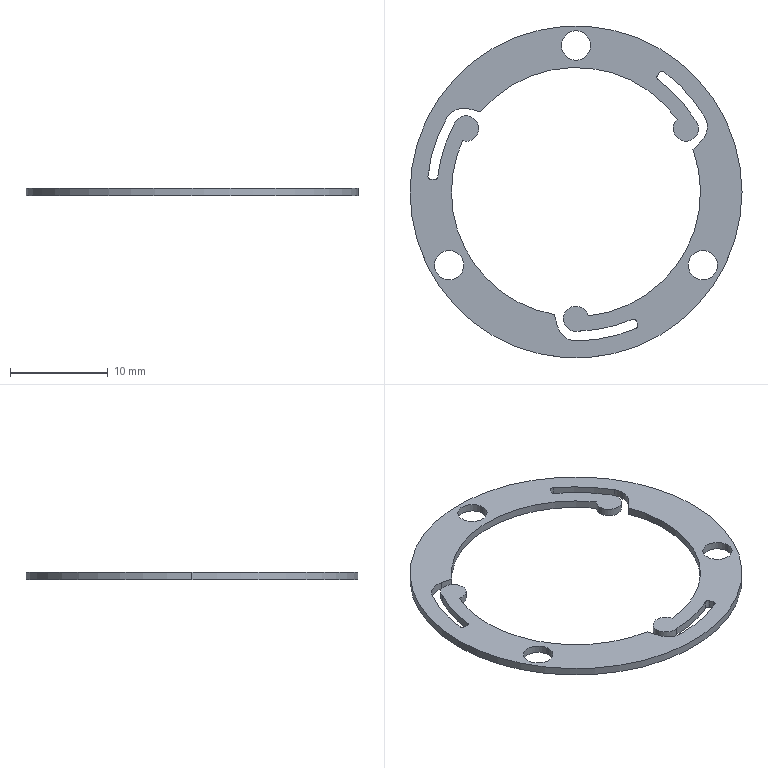Part | SolidWorks | features Fillet 3, ICE 3, CirPattern 2, DelFace 1, Extrusion 1 | 1 solid | 43 faces | box 34 x 34 x 0.8 mm | volume 283.992 mm3 | cylinder 35 | plane 8 | commonest cylinder face diameters 0.6 x7 2.6 x6 3 x6 4 x4 25.5 x4 28.5 x3
STEP:
#1=CARTESIAN_POINT('',(-17.,0.,0.));
#2=VERTEX_POINT('',#1);
#3=CARTESIAN_POINT('',(17.,0.,0.));
#4=VERTEX_POINT('',#3);
#5=CARTESIAN_POINT('',(0.,0.,0.));
#6=DIRECTION('',(0.,0.,-1.));
#7=DIRECTION('',(1.,0.,0.));
#8=AXIS2_PLACEMENT_3D('',#5,#6,#7);
#9=CIRCLE('',#8,17.);
#10=EDGE_CURVE('',#2,#4,#9,.T.);
#11=ORIENTED_EDGE('',*,*,#10,.F.);
#12=CARTESIAN_POINT('',(-17.,0.,0.8));
#13=VERTEX_POINT('',#12);
#14=CARTESIAN_POINT('',(-17.,0.,-26.154));
#15=DIRECTION('',(0.,0.,1.));
#16=VECTOR('',#15,1000.);
#17=LINE('',#14,#16);
#18=EDGE_CURVE('',#2,#13,#17,.T.);
#19=ORIENTED_EDGE('',*,*,#18,.T.);
#20=CARTESIAN_POINT('',(17.,0.,0.8));
#21=VERTEX_POINT('',#20);
#22=CARTESIAN_POINT('',(0.,0.,0.8));
#23=DIRECTION('',(0.,0.,1.));
#24=DIRECTION('',(1.,0.,0.));
#25=AXIS2_PLACEMENT_3D('',#22,#23,#24);
#26=CIRCLE('',#25,17.);
#27=EDGE_CURVE('',#21,#13,#26,.T.);
#28=ORIENTED_EDGE('',*,*,#27,.F.);
#29=CARTESIAN_POINT('',(17.,0.,-26.154));
#30=DIRECTION('',(0.,0.,1.));
#31=VECTOR('',#30,1000.);
#32=LINE('',#29,#31);
#33=EDGE_CURVE('',#4,#21,#32,.T.);
#34=ORIENTED_EDGE('',*,*,#33,.F.);
#35=EDGE_LOOP('',(#11,#19,#28,#34));
#36=FACE_OUTER_BOUND('',#35,.T.);
#37=CARTESIAN_POINT('',(0.,0.,-26.154));
#38=DIRECTION('',(0.,0.,1.));
#39=DIRECTION('',(1.,0.,0.));
#40=AXIS2_PLACEMENT_3D('',#37,#38,#39);
#41=CYLINDRICAL_SURFACE('',#40,17.);
#42=ADVANCED_FACE('',(#36),#41,.T.);
#43=CARTESIAN_POINT('',(6.345,-13.673,0.));
#44=VERTEX_POINT('',#43);
#45=CARTESIAN_POINT('',(6.317,-13.547,0.));
#46=VERTEX_POINT('',#45);
#47=CARTESIAN_POINT('',(6.045,-13.673,0.));
#48=DIRECTION('',(0.,0.,1.));
#49=DIRECTION('',(1.,0.,0.));
#50=AXIS2_PLACEMENT_3D('',#47,#48,#49);
#51=CIRCLE('',#50,0.3);
#52=EDGE_CURVE('',#44,#46,#51,.T.);
#53=ORIENTED_EDGE('',*,*,#52,.F.);
#54=CARTESIAN_POINT('',(6.345,-13.673,0.8));
#55=VERTEX_POINT('',#54);
#56=CARTESIAN_POINT('',(6.345,-13.673,-9.068));
#57=DIRECTION('',(0.,0.,1.));
#58=VECTOR('',#57,1000.);
#59=LINE('',#56,#58);
#60=EDGE_CURVE('',#44,#55,#59,.T.);
#61=ORIENTED_EDGE('',*,*,#60,.T.);
#62=CARTESIAN_POINT('',(6.317,-13.547,0.8));
#63=VERTEX_POINT('',#62);
#64=CARTESIAN_POINT('',(6.045,-13.673,0.8));
#65=DIRECTION('',(0.,0.,-1.));
#66=DIRECTION('',(1.,0.,0.));
#67=AXIS2_PLACEMENT_3D('',#64,#65,#66);
#68=CIRCLE('',#67,0.3);
#69=EDGE_CURVE('',#63,#55,#68,.T.);
#70=ORIENTED_EDGE('',*,*,#69,.F.);
#71=CARTESIAN_POINT('',(6.317,-13.547,0.8));
#72=DIRECTION('',(0.,0.,1.));
#73=VECTOR('',#72,1000.);
#74=LINE('',#71,#73);
#75=EDGE_CURVE('',#46,#63,#74,.T.);
#76=ORIENTED_EDGE('',*,*,#75,.F.);
#77=EDGE_LOOP('',(#53,#61,#70,#76));
#78=FACE_OUTER_BOUND('',#77,.T.);
#79=CARTESIAN_POINT('',(6.045,-13.673,-9.068));
#80=DIRECTION('',(0.,0.,1.));
#81=DIRECTION('',(1.,0.,0.));
#82=AXIS2_PLACEMENT_3D('',#79,#80,#81);
#83=CYLINDRICAL_SURFACE('',#82,0.3);
#84=ADVANCED_FACE('',(#78),#83,.F.);
#85=CARTESIAN_POINT('',(-9.958,6.5,0.));
#86=VERTEX_POINT('',#85);
#87=CARTESIAN_POINT('',(-11.619,5.251,0.));
#88=VERTEX_POINT('',#87);
#89=CARTESIAN_POINT('',(-11.258,6.5,0.));
#90=DIRECTION('',(0.,0.,-1.));
#91=DIRECTION('',(1.,0.,0.));
#92=AXIS2_PLACEMENT_3D('',#89,#90,#91);
#93=CIRCLE('',#92,1.3);
#94=EDGE_CURVE('',#86,#88,#93,.T.);
#95=ORIENTED_EDGE('',*,*,#94,.F.);
#96=CARTESIAN_POINT('',(-9.958,6.5,0.8));
#97=VERTEX_POINT('',#96);
#98=CARTESIAN_POINT('',(-9.958,6.5,-3.677));
#99=DIRECTION('',(0.,0.,1.));
#100=VECTOR('',#99,1000.);
#101=LINE('',#98,#100);
#102=EDGE_CURVE('',#86,#97,#101,.T.);
#103=ORIENTED_EDGE('',*,*,#102,.T.);
#104=CARTESIAN_POINT('',(-11.619,5.251,0.8));
#105=VERTEX_POINT('',#104);
#106=CARTESIAN_POINT('',(-11.258,6.5,0.8));
#107=DIRECTION('',(0.,0.,1.));
#108=DIRECTION('',(-0.5,0.866,0.));
#109=AXIS2_PLACEMENT_3D('',#106,#107,#108);
#110=CIRCLE('',#109,1.3);
#111=EDGE_CURVE('',#105,#97,#110,.T.);
#112=ORIENTED_EDGE('',*,*,#111,.F.);
#113=CARTESIAN_POINT('',(-11.619,5.251,0.4));
#114=DIRECTION('',(0.,0.,-1.));
#115=VECTOR('',#114,1000.);
#116=LINE('',#113,#115);
#117=EDGE_CURVE('',#105,#88,#116,.T.);
#118=ORIENTED_EDGE('',*,*,#117,.T.);
#119=EDGE_LOOP('',(#95,#103,#112,#118));
#120=FACE_OUTER_BOUND('',#119,.T.);
#121=CARTESIAN_POINT('',(-11.258,6.5,-3.677));
#122=DIRECTION('',(0.,0.,1.));
#123=DIRECTION('',(1.,0.,0.));
#124=AXIS2_PLACEMENT_3D('',#121,#122,#123);
#125=CYLINDRICAL_SURFACE('',#124,1.3);
#126=ADVANCED_FACE('',(#120),#125,.T.);
#127=CARTESIAN_POINT('',(9.958,6.5,0.));
#128=VERTEX_POINT('',#127);
#129=CARTESIAN_POINT('',(10.357,7.437,0.));
#130=VERTEX_POINT('',#129);
#131=CARTESIAN_POINT('',(11.258,6.5,0.));
#132=DIRECTION('',(0.,0.,-1.));
#133=DIRECTION('',(1.,0.,0.));
#134=AXIS2_PLACEMENT_3D('',#131,#132,#133);
#135=CIRCLE('',#134,1.3);
#136=EDGE_CURVE('',#128,#130,#135,.T.);
#137=ORIENTED_EDGE('',*,*,#136,.F.);
#138=CARTESIAN_POINT('',(9.958,6.5,0.8));
#139=VERTEX_POINT('',#138);
#140=CARTESIAN_POINT('',(9.958,6.5,-3.677));
#141=DIRECTION('',(0.,0.,1.));
#142=VECTOR('',#141,1000.);
#143=LINE('',#140,#142);
#144=EDGE_CURVE('',#128,#139,#143,.T.);
#145=ORIENTED_EDGE('',*,*,#144,.T.);
#146=CARTESIAN_POINT('',(10.357,7.437,0.8));
#147=VERTEX_POINT('',#146);
#148=CARTESIAN_POINT('',(11.258,6.5,0.8));
#149=DIRECTION('',(0.,0.,1.));
#150=DIRECTION('',(1.,0.,0.));
#151=AXIS2_PLACEMENT_3D('',#148,#149,#150);
#152=CIRCLE('',#151,1.3);
#153=EDGE_CURVE('',#147,#139,#152,.T.);
#154=ORIENTED_EDGE('',*,*,#153,.F.);
#155=CARTESIAN_POINT('',(10.357,7.437,0.4));
#156=DIRECTION('',(0.,0.,-1.));
#157=VECTOR('',#156,1000.);
#158=LINE('',#155,#157);
#159=EDGE_CURVE('',#147,#130,#158,.T.);
#160=ORIENTED_EDGE('',*,*,#159,.T.);
#161=EDGE_LOOP('',(#137,#145,#154,#160));
#162=FACE_OUTER_BOUND('',#161,.T.);
#163=CARTESIAN_POINT('',(11.258,6.5,-3.677));
#164=DIRECTION('',(0.,0.,1.));
#165=DIRECTION('',(1.,0.,0.));
#166=AXIS2_PLACEMENT_3D('',#163,#164,#165);
#167=CYLINDRICAL_SURFACE('',#166,1.3);
#168=ADVANCED_FACE('',(#162),#167,.T.);
#169=ORIENTED_EDGE('',*,*,#144,.F.);
#170=CARTESIAN_POINT('',(12.558,6.5,0.));
#171=VERTEX_POINT('',#170);
#172=CARTESIAN_POINT('',(11.258,6.5,0.));
#173=DIRECTION('',(0.,0.,-1.));
#174=DIRECTION('',(1.,0.,0.));
#175=AXIS2_PLACEMENT_3D('',#172,#173,#174);
#176=CIRCLE('',#175,1.3);
#177=EDGE_CURVE('',#171,#128,#176,.T.);
#178=ORIENTED_EDGE('',*,*,#177,.F.);
#179=CARTESIAN_POINT('',(12.558,6.5,0.8));
#180=VERTEX_POINT('',#179);
#181=CARTESIAN_POINT('',(12.558,6.5,-3.677));
#182=DIRECTION('',(0.,0.,1.));
#183=VECTOR('',#182,1000.);
#184=LINE('',#181,#183);
#185=EDGE_CURVE('',#171,#180,#184,.T.);
#186=ORIENTED_EDGE('',*,*,#185,.T.);
#187=CARTESIAN_POINT('',(11.258,6.5,0.8));
#188=DIRECTION('',(0.,0.,1.));
#189=DIRECTION('',(1.,0.,0.));
#190=AXIS2_PLACEMENT_3D('',#187,#188,#189);
#191=CIRCLE('',#190,1.3);
#192=EDGE_CURVE('',#139,#180,#191,.T.);
#193=ORIENTED_EDGE('',*,*,#192,.F.);
#194=EDGE_LOOP('',(#169,#178,#186,#193));
#195=FACE_OUTER_BOUND('',#194,.T.);
#196=CARTESIAN_POINT('',(11.258,6.5,-3.677));
#197=DIRECTION('',(0.,0.,1.));
#198=DIRECTION('',(1.,0.,0.));
#199=AXIS2_PLACEMENT_3D('',#196,#197,#198);
#200=CYLINDRICAL_SURFACE('',#199,1.3);
#201=ADVANCED_FACE('',(#195),#200,.T.);
#202=CARTESIAN_POINT('',(13.454,6.662,0.));
#203=VERTEX_POINT('',#202);
#204=CARTESIAN_POINT('',(13.182,7.667,0.));
#205=VERTEX_POINT('',#204);
#206=CARTESIAN_POINT('',(11.454,6.662,0.));
#207=DIRECTION('',(0.,0.,1.));
#208=DIRECTION('',(1.,0.,0.));
#209=AXIS2_PLACEMENT_3D('',#206,#207,#208);
#210=CIRCLE('',#209,2.);
#211=EDGE_CURVE('',#203,#205,#210,.T.);
#212=ORIENTED_EDGE('',*,*,#211,.F.);
#213=CARTESIAN_POINT('',(13.454,6.662,0.8));
#214=VERTEX_POINT('',#213);
#215=CARTESIAN_POINT('',(13.454,6.662,-9.944));
#216=DIRECTION('',(0.,0.,1.));
#217=VECTOR('',#216,1000.);
#218=LINE('',#215,#217);
#219=EDGE_CURVE('',#203,#214,#218,.T.);
#220=ORIENTED_EDGE('',*,*,#219,.T.);
#221=CARTESIAN_POINT('',(13.182,7.667,0.8));
#222=VERTEX_POINT('',#221);
#223=CARTESIAN_POINT('',(11.454,6.662,0.8));
#224=DIRECTION('',(0.,0.,-1.));
#225=DIRECTION('',(1.,0.,0.));
#226=AXIS2_PLACEMENT_3D('',#223,#224,#225);
#227=CIRCLE('',#226,2.);
#228=EDGE_CURVE('',#222,#214,#227,.T.);
#229=ORIENTED_EDGE('',*,*,#228,.F.);
#230=CARTESIAN_POINT('',(13.182,7.667,-9.944));
#231=DIRECTION('',(0.,0.,1.));
#232=VECTOR('',#231,1000.);
#233=LINE('',#230,#232);
#234=EDGE_CURVE('',#205,#222,#233,.T.);
#235=ORIENTED_EDGE('',*,*,#234,.F.);
#236=EDGE_LOOP('',(#212,#220,#229,#235));
#237=FACE_OUTER_BOUND('',#236,.T.);
#238=CARTESIAN_POINT('',(11.454,6.662,-9.944));
#239=DIRECTION('',(0.,0.,1.));
#240=DIRECTION('',(1.,0.,0.));
#241=AXIS2_PLACEMENT_3D('',#238,#239,#240);
#242=CYLINDRICAL_SURFACE('',#241,2.);
#243=ADVANCED_FACE('',(#237),#242,.F.);
#244=CARTESIAN_POINT('',(-14.49,-7.5,0.8));
#245=VERTEX_POINT('',#244);
#246=CARTESIAN_POINT('',(-11.49,-7.5,0.8));
#247=VERTEX_POINT('',#246);
#248=CARTESIAN_POINT('',(-12.99,-7.5,0.8));
#249=DIRECTION('',(0.,0.,1.));
#250=DIRECTION('',(1.,0.,0.));
#251=AXIS2_PLACEMENT_3D('',#248,#249,#250);
#252=CIRCLE('',#251,1.5);
#253=EDGE_CURVE('',#245,#247,#252,.T.);
#254=ORIENTED_EDGE('',*,*,#253,.T.);
#255=CARTESIAN_POINT('',(-11.49,-7.5,0.));
#256=VERTEX_POINT('',#255);
#257=CARTESIAN_POINT('',(-11.49,-7.5,0.8));
#258=DIRECTION('',(0.,0.,-1.));
#259=VECTOR('',#258,1000.);
#260=LINE('',#257,#259);
#261=EDGE_CURVE('',#247,#256,#260,.T.);
#262=ORIENTED_EDGE('',*,*,#261,.T.);
#263=CARTESIAN_POINT('',(-14.49,-7.5,0.));
#264=VERTEX_POINT('',#263);
#265=CARTESIAN_POINT('',(-12.99,-7.5,0.));
#266=DIRECTION('',(0.,0.,1.));
#267=DIRECTION('',(1.,0.,0.));
#268=AXIS2_PLACEMENT_3D('',#265,#266,#267);
#269=CIRCLE('',#268,1.5);
#270=EDGE_CURVE('',#264,#256,#269,.T.);
#271=ORIENTED_EDGE('',*,*,#270,.F.);
#272=CARTESIAN_POINT('',(-14.49,-7.5,0.8));
#273=DIRECTION('',(0.,0.,-1.));
#274=VECTOR('',#273,1000.);
#275=LINE('',#272,#274);
#276=EDGE_CURVE('',#245,#264,#275,.T.);
#277=ORIENTED_EDGE('',*,*,#276,.F.);
#278=EDGE_LOOP('',(#254,#262,#271,#277));
#279=FACE_OUTER_BOUND('',#278,.T.);
#280=CARTESIAN_POINT('',(-12.99,-7.5,0.8));
#281=DIRECTION('',(0.,0.,-1.));
#282=DIRECTION('',(-1.,0.,0.));
#283=AXIS2_PLACEMENT_3D('',#280,#281,#282);
#284=CYLINDRICAL_SURFACE('',#283,1.5);
#285=ADVANCED_FACE('',(#279),#284,.F.);
#286=CARTESIAN_POINT('',(11.49,-7.5,0.8));
#287=VERTEX_POINT('',#286);
#288=CARTESIAN_POINT('',(14.49,-7.5,0.8));
#289=VERTEX_POINT('',#288);
#290=CARTESIAN_POINT('',(12.99,-7.5,0.8));
#291=DIRECTION('',(0.,0.,1.));
#292=DIRECTION('',(1.,0.,0.));
#293=AXIS2_PLACEMENT_3D('',#290,#291,#292);
#294=CIRCLE('',#293,1.5);
#295=EDGE_CURVE('',#287,#289,#294,.T.);
#296=ORIENTED_EDGE('',*,*,#295,.T.);
#297=CARTESIAN_POINT('',(14.49,-7.5,0.));
#298=VERTEX_POINT('',#297);
#299=CARTESIAN_POINT('',(14.49,-7.5,0.8));
#300=DIRECTION('',(0.,0.,-1.));
#301=VECTOR('',#300,1000.);
#302=LINE('',#299,#301);
#303=EDGE_CURVE('',#289,#298,#302,.T.);
#304=ORIENTED_EDGE('',*,*,#303,.T.);
#305=CARTESIAN_POINT('',(11.49,-7.5,0.));
#306=VERTEX_POINT('',#305);
#307=CARTESIAN_POINT('',(12.99,-7.5,0.));
#308=DIRECTION('',(0.,0.,1.));
#309=DIRECTION('',(1.,0.,0.));
#310=AXIS2_PLACEMENT_3D('',#307,#308,#309);
#311=CIRCLE('',#310,1.5);
#312=EDGE_CURVE('',#306,#298,#311,.T.);
#313=ORIENTED_EDGE('',*,*,#312,.F.);
#314=CARTESIAN_POINT('',(11.49,-7.5,0.8));
#315=DIRECTION('',(0.,0.,-1.));
#316=VECTOR('',#315,1000.);
#317=LINE('',#314,#316);
#318=EDGE_CURVE('',#287,#306,#317,.T.);
#319=ORIENTED_EDGE('',*,*,#318,.F.);
#320=EDGE_LOOP('',(#296,#304,#313,#319));
#321=FACE_OUTER_BOUND('',#320,.T.);
#322=CARTESIAN_POINT('',(12.99,-7.5,0.8));
#323=DIRECTION('',(0.,0.,-1.));
#324=DIRECTION('',(-1.,0.,0.));
#325=AXIS2_PLACEMENT_3D('',#322,#323,#324);
#326=CYLINDRICAL_SURFACE('',#325,1.5);
#327=ADVANCED_FACE('',(#321),#326,.F.);
#328=CARTESIAN_POINT('',(-1.5,15.,0.8));
#329=VERTEX_POINT('',#328);
#330=CARTESIAN_POINT('',(1.5,15.,0.8));
#331=VERTEX_POINT('',#330);
#332=CARTESIAN_POINT('',(0.,15.,0.8));
#333=DIRECTION('',(0.,0.,1.));
#334=DIRECTION('',(1.,0.,0.));
#335=AXIS2_PLACEMENT_3D('',#332,#333,#334);
#336=CIRCLE('',#335,1.5);
#337=EDGE_CURVE('',#329,#331,#336,.T.);
#338=ORIENTED_EDGE('',*,*,#337,.T.);
#339=CARTESIAN_POINT('',(1.5,15.,0.));
#340=VERTEX_POINT('',#339);
#341=CARTESIAN_POINT('',(1.5,15.,0.8));
#342=DIRECTION('',(0.,0.,-1.));
#343=VECTOR('',#342,1000.);
#344=LINE('',#341,#343);
#345=EDGE_CURVE('',#331,#340,#344,.T.);
#346=ORIENTED_EDGE('',*,*,#345,.T.);
#347=CARTESIAN_POINT('',(-1.5,15.,0.));
#348=VERTEX_POINT('',#347);
#349=CARTESIAN_POINT('',(0.,15.,0.));
#350=DIRECTION('',(0.,0.,1.));
#351=DIRECTION('',(1.,0.,0.));
#352=AXIS2_PLACEMENT_3D('',#349,#350,#351);
#353=CIRCLE('',#352,1.5);
#354=EDGE_CURVE('',#348,#340,#353,.T.);
#355=ORIENTED_EDGE('',*,*,#354,.F.);
#356=CARTESIAN_POINT('',(-1.5,15.,0.8));
#357=DIRECTION('',(0.,0.,-1.));
#358=VECTOR('',#357,1000.);
#359=LINE('',#356,#358);
#360=EDGE_CURVE('',#329,#348,#359,.T.);
#361=ORIENTED_EDGE('',*,*,#360,.F.);
#362=EDGE_LOOP('',(#338,#346,#355,#361));
#363=FACE_OUTER_BOUND('',#362,.T.);
#364=CARTESIAN_POINT('',(0.,15.,0.8));
#365=DIRECTION('',(0.,0.,-1.));
#366=DIRECTION('',(-1.,0.,0.));
#367=AXIS2_PLACEMENT_3D('',#364,#365,#366);
#368=CYLINDRICAL_SURFACE('',#367,1.5);
#369=ADVANCED_FACE('',(#363),#368,.F.);
#370=CARTESIAN_POINT('',(-12.75,0.,0.8));
#371=VERTEX_POINT('',#370);
#372=CARTESIAN_POINT('',(0.,0.,0.8));
#373=DIRECTION('',(0.,0.,1.));
#374=DIRECTION('',(1.,0.,0.));
#375=AXIS2_PLACEMENT_3D('',#372,#373,#374);
#376=CIRCLE('',#375,12.75);
#377=EDGE_CURVE('',#105,#371,#376,.T.);
#378=ORIENTED_EDGE('',*,*,#377,.T.);
#379=CARTESIAN_POINT('',(-12.75,0.,0.));
#380=VERTEX_POINT('',#379);
#381=CARTESIAN_POINT('',(-12.75,0.,0.8));
#382=DIRECTION('',(0.,0.,-1.));
#383=VECTOR('',#382,1000.);
#384=LINE('',#381,#383);
#385=EDGE_CURVE('',#371,#380,#384,.T.);
#386=ORIENTED_EDGE('',*,*,#385,.T.);
#387=CARTESIAN_POINT('',(0.,0.,0.));
#388=DIRECTION('',(0.,0.,1.));
#389=DIRECTION('',(1.,0.,0.));
#390=AXIS2_PLACEMENT_3D('',#387,#388,#389);
#391=CIRCLE('',#390,12.75);
#392=EDGE_CURVE('',#88,#380,#391,.T.);
#393=ORIENTED_EDGE('',*,*,#392,.F.);
#394=ORIENTED_EDGE('',*,*,#117,.F.);
#395=EDGE_LOOP('',(#378,#386,#393,#394));
#396=FACE_OUTER_BOUND('',#395,.T.);
#397=CARTESIAN_POINT('',(0.,0.,0.8));
#398=DIRECTION('',(0.,0.,-1.));
#399=DIRECTION('',(-1.,0.,0.));
#400=AXIS2_PLACEMENT_3D('',#397,#398,#399);
#401=CYLINDRICAL_SURFACE('',#400,12.75);
#402=ADVANCED_FACE('',(#396),#401,.F.);
#403=CARTESIAN_POINT('',(1.262,-12.687,0.8));
#404=VERTEX_POINT('',#403);
#405=CARTESIAN_POINT('',(11.981,4.361,0.8));
#406=VERTEX_POINT('',#405);
#407=CARTESIAN_POINT('',(0.,0.,0.8));
#408=DIRECTION('',(0.,0.,1.));
#409=DIRECTION('',(1.,0.,0.));
#410=AXIS2_PLACEMENT_3D('',#407,#408,#409);
#411=CIRCLE('',#410,12.75);
#412=EDGE_CURVE('',#404,#406,#411,.T.);
#413=ORIENTED_EDGE('',*,*,#412,.F.);
#414=CARTESIAN_POINT('',(0.3738,-14.245,0.8));
#415=VERTEX_POINT('',#414);
#416=CARTESIAN_POINT('',(0.,-13.,0.8));
#417=DIRECTION('',(0.,0.,1.));
#418=DIRECTION('',(-0.5,-0.866,0.));
#419=AXIS2_PLACEMENT_3D('',#416,#417,#418);
#420=CIRCLE('',#419,1.3);
#421=EDGE_CURVE('',#404,#415,#420,.T.);
#422=ORIENTED_EDGE('',*,*,#421,.T.);
#423=CARTESIAN_POINT('',(5.755,-13.036,0.8));
#424=VERTEX_POINT('',#423);
#425=CARTESIAN_POINT('',(0.,0.,0.8));
#426=DIRECTION('',(0.,0.,-1.));
#427=DIRECTION('',(-0.5,-0.866,0.));
#428=AXIS2_PLACEMENT_3D('',#425,#426,#427);
#429=CIRCLE('',#428,14.25);
#430=EDGE_CURVE('',#424,#415,#429,.T.);
#431=ORIENTED_EDGE('',*,*,#430,.F.);
#432=CARTESIAN_POINT('',(6.148,-13.184,0.8));
#433=VERTEX_POINT('',#432);
#434=CARTESIAN_POINT('',(5.876,-13.311,0.8));
#435=DIRECTION('',(0.,0.,-1.));
#436=DIRECTION('',(1.,0.,0.));
#437=AXIS2_PLACEMENT_3D('',#434,#435,#436);
#438=CIRCLE('',#437,0.3);
#439=EDGE_CURVE('',#424,#433,#438,.T.);
#440=ORIENTED_EDGE('',*,*,#439,.T.);
#441=CARTESIAN_POINT('',(6.445,-13.821,0.8));
#442=DIRECTION('',(-0.4226,0.9063,0.));
#443=VECTOR('',#442,1000.);
#444=LINE('',#441,#443);
#445=EDGE_CURVE('',#63,#433,#444,.T.);
#446=ORIENTED_EDGE('',*,*,#445,.F.);
#447=ORIENTED_EDGE('',*,*,#69,.T.);
#448=CARTESIAN_POINT('',(6.166,-13.948,0.8));
#449=VERTEX_POINT('',#448);
#450=CARTESIAN_POINT('',(6.045,-13.673,0.8));
#451=DIRECTION('',(0.,0.,-1.));
#452=DIRECTION('',(1.,0.,0.));
#453=AXIS2_PLACEMENT_3D('',#450,#451,#452);
#454=CIRCLE('',#453,0.3);
#455=EDGE_CURVE('',#55,#449,#454,.T.);
#456=ORIENTED_EDGE('',*,*,#455,.T.);
#457=CARTESIAN_POINT('',(0.0488,-15.25,0.8));
#458=VERTEX_POINT('',#457);
#459=CARTESIAN_POINT('',(0.,0.,0.8));
#460=DIRECTION('',(0.,0.,1.));
#461=DIRECTION('',(-0.5,-0.866,0.));
#462=AXIS2_PLACEMENT_3D('',#459,#460,#461);
#463=CIRCLE('',#462,15.25);
#464=EDGE_CURVE('',#458,#449,#463,.T.);
#465=ORIENTED_EDGE('',*,*,#464,.F.);
#466=CARTESIAN_POINT('',(-1.889,-13.768,0.8));
#467=VERTEX_POINT('',#466);
#468=CARTESIAN_POINT('',(0.0424,-13.25,0.8));
#469=DIRECTION('',(0.,0.,-1.));
#470=DIRECTION('',(1.,0.,0.));
#471=AXIS2_PLACEMENT_3D('',#468,#469,#470);
#472=CIRCLE('',#471,2.);
#473=EDGE_CURVE('',#458,#467,#472,.T.);
#474=ORIENTED_EDGE('',*,*,#473,.T.);
#475=CARTESIAN_POINT('',(-2.214,-12.556,0.8));
#476=VERTEX_POINT('',#475);
#477=CARTESIAN_POINT('',(-2.214,-12.556,0.8));
#478=DIRECTION('',(0.2588,-0.9659,0.));
#479=VECTOR('',#478,1000.);
#480=LINE('',#477,#479);
#481=EDGE_CURVE('',#476,#467,#480,.T.);
#482=ORIENTED_EDGE('',*,*,#481,.F.);
#483=CARTESIAN_POINT('',(0.,0.,0.8));
#484=DIRECTION('',(0.,0.,1.));
#485=DIRECTION('',(1.,0.,0.));
#486=AXIS2_PLACEMENT_3D('',#483,#484,#485);
#487=CIRCLE('',#486,12.75);
#488=EDGE_CURVE('',#371,#476,#487,.T.);
#489=ORIENTED_EDGE('',*,*,#488,.F.);
#490=ORIENTED_EDGE('',*,*,#377,.F.);
#491=ORIENTED_EDGE('',*,*,#111,.T.);
#492=CARTESIAN_POINT('',(-12.524,6.799,0.8));
#493=VERTEX_POINT('',#492);
#494=CARTESIAN_POINT('',(-11.258,6.5,0.8));
#495=DIRECTION('',(0.,0.,1.));
#496=DIRECTION('',(-0.5,0.866,0.));
#497=AXIS2_PLACEMENT_3D('',#494,#495,#496);
#498=CIRCLE('',#497,1.3);
#499=EDGE_CURVE('',#97,#493,#498,.T.);
#500=ORIENTED_EDGE('',*,*,#499,.T.);
#501=CARTESIAN_POINT('',(-14.167,1.534,0.8));
#502=VERTEX_POINT('',#501);
#503=CARTESIAN_POINT('',(0.,0.,0.8));
#504=DIRECTION('',(0.,0.,-1.));
#505=DIRECTION('',(-0.5,0.866,0.));
#506=AXIS2_PLACEMENT_3D('',#503,#504,#505);
#507=CIRCLE('',#506,14.25);
#508=EDGE_CURVE('',#502,#493,#507,.T.);
#509=ORIENTED_EDGE('',*,*,#508,.F.);
#510=CARTESIAN_POINT('',(-14.492,1.268,0.8));
#511=VERTEX_POINT('',#510);
#512=CARTESIAN_POINT('',(-14.465,1.567,0.8));
#513=DIRECTION('',(0.,0.,-1.));
#514=DIRECTION('',(1.,0.,0.));
#515=AXIS2_PLACEMENT_3D('',#512,#513,#514);
#516=CIRCLE('',#515,0.3);
#517=EDGE_CURVE('',#502,#511,#516,.T.);
#518=ORIENTED_EDGE('',*,*,#517,.T.);
#519=CARTESIAN_POINT('',(-14.89,1.303,0.8));
#520=VERTEX_POINT('',#519);
#521=CARTESIAN_POINT('',(-15.192,1.329,0.8));
#522=DIRECTION('',(0.9962,-0.08716,0.));
#523=VECTOR('',#522,1000.);
#524=LINE('',#521,#523);
#525=EDGE_CURVE('',#520,#511,#524,.T.);
#526=ORIENTED_EDGE('',*,*,#525,.F.);
#527=CARTESIAN_POINT('',(-15.162,1.634,0.8));
#528=VERTEX_POINT('',#527);
#529=CARTESIAN_POINT('',(-14.864,1.602,0.8));
#530=DIRECTION('',(0.,0.,-1.));
#531=DIRECTION('',(1.,0.,0.));
#532=AXIS2_PLACEMENT_3D('',#529,#530,#531);
#533=CIRCLE('',#532,0.3);
#534=EDGE_CURVE('',#520,#528,#533,.T.);
#535=ORIENTED_EDGE('',*,*,#534,.T.);
#536=CARTESIAN_POINT('',(-13.231,7.583,0.8));
#537=VERTEX_POINT('',#536);
#538=CARTESIAN_POINT('',(0.,0.,0.8));
#539=DIRECTION('',(0.,0.,1.));
#540=DIRECTION('',(-0.5,0.866,0.));
#541=AXIS2_PLACEMENT_3D('',#538,#539,#540);
#542=CIRCLE('',#541,15.25);
#543=EDGE_CURVE('',#537,#528,#542,.T.);
#544=ORIENTED_EDGE('',*,*,#543,.F.);
#545=CARTESIAN_POINT('',(-10.978,8.52,0.8));
#546=VERTEX_POINT('',#545);
#547=CARTESIAN_POINT('',(-11.496,6.588,0.8));
#548=DIRECTION('',(0.,0.,-1.));
#549=DIRECTION('',(1.,0.,0.));
#550=AXIS2_PLACEMENT_3D('',#547,#548,#549);
#551=CIRCLE('',#550,2.);
#552=EDGE_CURVE('',#537,#546,#551,.T.);
#553=ORIENTED_EDGE('',*,*,#552,.T.);
#554=CARTESIAN_POINT('',(-9.767,8.196,0.8));
#555=VERTEX_POINT('',#554);
#556=CARTESIAN_POINT('',(-9.767,8.196,0.8));
#557=DIRECTION('',(-0.9659,0.2588,0.));
#558=VECTOR('',#557,1000.);
#559=LINE('',#556,#558);
#560=EDGE_CURVE('',#555,#546,#559,.T.);
#561=ORIENTED_EDGE('',*,*,#560,.F.);
#562=CARTESIAN_POINT('',(0.,0.,0.8));
#563=DIRECTION('',(0.,0.,1.));
#564=DIRECTION('',(1.,0.,0.));
#565=AXIS2_PLACEMENT_3D('',#562,#563,#564);
#566=CIRCLE('',#565,12.75);
#567=EDGE_CURVE('',#147,#555,#566,.T.);
#568=ORIENTED_EDGE('',*,*,#567,.F.);
#569=ORIENTED_EDGE('',*,*,#153,.T.);
#570=ORIENTED_EDGE('',*,*,#192,.T.);
#571=CARTESIAN_POINT('',(12.15,7.446,0.8));
#572=VERTEX_POINT('',#571);
#573=CARTESIAN_POINT('',(11.258,6.5,0.8));
#574=DIRECTION('',(0.,0.,1.));
#575=DIRECTION('',(1.,0.,0.));
#576=AXIS2_PLACEMENT_3D('',#573,#574,#575);
#577=CIRCLE('',#576,1.3);
#578=EDGE_CURVE('',#180,#572,#577,.T.);
#579=ORIENTED_EDGE('',*,*,#578,.T.);
#580=CARTESIAN_POINT('',(8.412,11.502,0.8));
#581=VERTEX_POINT('',#580);
#582=CARTESIAN_POINT('',(0.,0.,0.8));
#583=DIRECTION('',(0.,0.,-1.));
#584=DIRECTION('',(1.,0.,0.));
#585=AXIS2_PLACEMENT_3D('',#582,#583,#584);
#586=CIRCLE('',#585,14.25);
#587=EDGE_CURVE('',#581,#572,#586,.T.);
#588=ORIENTED_EDGE('',*,*,#587,.F.);
#589=CARTESIAN_POINT('',(8.344,11.916,0.8));
#590=VERTEX_POINT('',#589);
#591=CARTESIAN_POINT('',(8.59,11.744,0.8));
#592=DIRECTION('',(0.,0.,-1.));
#593=DIRECTION('',(1.,0.,0.));
#594=AXIS2_PLACEMENT_3D('',#591,#592,#593);
#595=CIRCLE('',#594,0.3);
#596=EDGE_CURVE('',#581,#590,#595,.T.);
#597=ORIENTED_EDGE('',*,*,#596,.T.);
#598=CARTESIAN_POINT('',(8.573,12.244,0.8));
#599=VERTEX_POINT('',#598);
#600=CARTESIAN_POINT('',(8.747,12.492,0.8));
#601=DIRECTION('',(-0.5736,-0.8192,0.));
#602=VECTOR('',#601,1000.);
#603=LINE('',#600,#602);
#604=EDGE_CURVE('',#599,#590,#603,.T.);
#605=ORIENTED_EDGE('',*,*,#604,.F.);
#606=CARTESIAN_POINT('',(8.996,12.314,0.8));
#607=VERTEX_POINT('',#606);
#608=CARTESIAN_POINT('',(8.819,12.072,0.8));
#609=DIRECTION('',(0.,0.,-1.));
#610=DIRECTION('',(1.,0.,0.));
#611=AXIS2_PLACEMENT_3D('',#608,#609,#610);
#612=CIRCLE('',#611,0.3);
#613=EDGE_CURVE('',#599,#607,#612,.T.);
#614=ORIENTED_EDGE('',*,*,#613,.T.);
#615=CARTESIAN_POINT('',(0.,0.,0.8));
#616=DIRECTION('',(0.,0.,1.));
#617=DIRECTION('',(1.,0.,0.));
#618=AXIS2_PLACEMENT_3D('',#615,#616,#617);
#619=CIRCLE('',#618,15.25);
#620=EDGE_CURVE('',#222,#607,#619,.T.);
#621=ORIENTED_EDGE('',*,*,#620,.F.);
#622=ORIENTED_EDGE('',*,*,#228,.T.);
#623=CARTESIAN_POINT('',(12.868,5.247,0.8));
#624=VERTEX_POINT('',#623);
#625=CARTESIAN_POINT('',(11.454,6.662,0.8));
#626=DIRECTION('',(0.,0.,-1.));
#627=DIRECTION('',(1.,0.,0.));
#628=AXIS2_PLACEMENT_3D('',#625,#626,#627);
#629=CIRCLE('',#628,2.);
#630=EDGE_CURVE('',#214,#624,#629,.T.);
#631=ORIENTED_EDGE('',*,*,#630,.T.);
#632=CARTESIAN_POINT('',(11.981,4.361,0.8));
#633=DIRECTION('',(0.7071,0.7071,0.));
#634=VECTOR('',#633,1000.);
#635=LINE('',#632,#634);
#636=EDGE_CURVE('',#406,#624,#635,.T.);
#637=ORIENTED_EDGE('',*,*,#636,.F.);
#638=EDGE_LOOP('',(#413,#422,#431,#440,#446,#447,#456,#465,#474,#482,#489,#490,#491,#500,#509,#518,#526,#535,#544,#553,#561,#568,#569,#570,#579,#588,#597,#605,#614,#621,#622,#631,#637));
#639=FACE_BOUND('',#638,.T.);
#640=ORIENTED_EDGE('',*,*,#295,.F.);
#641=CARTESIAN_POINT('',(12.99,-7.5,0.8));
#642=DIRECTION('',(0.,0.,1.));
#643=DIRECTION('',(1.,0.,0.));
#644=AXIS2_PLACEMENT_3D('',#641,#642,#643);
#645=CIRCLE('',#644,1.5);
#646=EDGE_CURVE('',#289,#287,#645,.T.);
#647=ORIENTED_EDGE('',*,*,#646,.F.);
#648=EDGE_LOOP('',(#640,#647));
#649=FACE_BOUND('',#648,.T.);
#650=ORIENTED_EDGE('',*,*,#337,.F.);
#651=CARTESIAN_POINT('',(0.,15.,0.8));
#652=DIRECTION('',(0.,0.,1.));
#653=DIRECTION('',(1.,0.,0.));
#654=AXIS2_PLACEMENT_3D('',#651,#652,#653);
#655=CIRCLE('',#654,1.5);
#656=EDGE_CURVE('',#331,#329,#655,.T.);
#657=ORIENTED_EDGE('',*,*,#656,.F.);
#658=EDGE_LOOP('',(#650,#657));
#659=FACE_BOUND('',#658,.T.);
#660=ORIENTED_EDGE('',*,*,#253,.F.);
#661=CARTESIAN_POINT('',(-12.99,-7.5,0.8));
#662=DIRECTION('',(0.,0.,1.));
#663=DIRECTION('',(1.,0.,0.));
#664=AXIS2_PLACEMENT_3D('',#661,#662,#663);
#665=CIRCLE('',#664,1.5);
#666=EDGE_CURVE('',#247,#245,#665,.T.);
#667=ORIENTED_EDGE('',*,*,#666,.F.);
#668=EDGE_LOOP('',(#660,#667));
#669=FACE_BOUND('',#668,.T.);
#670=ORIENTED_EDGE('',*,*,#27,.T.);
#671=CARTESIAN_POINT('',(0.,0.,0.8));
#672=DIRECTION('',(0.,0.,1.));
#673=DIRECTION('',(1.,0.,0.));
#674=AXIS2_PLACEMENT_3D('',#671,#672,#673);
#675=CIRCLE('',#674,17.);
#676=EDGE_CURVE('',#13,#21,#675,.T.);
#677=ORIENTED_EDGE('',*,*,#676,.T.);
#678=EDGE_LOOP('',(#670,#677));
#679=FACE_OUTER_BOUND('',#678,.T.);
#680=CARTESIAN_POINT('',(0.,0.,0.8));
#681=DIRECTION('',(0.,0.,1.));
#682=DIRECTION('',(1.,0.,0.));
#683=AXIS2_PLACEMENT_3D('',#680,#681,#682);
#684=PLANE('',#683);
#685=ADVANCED_FACE('',(#639,#649,#659,#669,#679),#684,.T.);
#686=ORIENTED_EDGE('',*,*,#270,.T.);
#687=CARTESIAN_POINT('',(-12.99,-7.5,0.));
#688=DIRECTION('',(0.,0.,1.));
#689=DIRECTION('',(1.,0.,0.));
#690=AXIS2_PLACEMENT_3D('',#687,#688,#689);
#691=CIRCLE('',#690,1.5);
#692=EDGE_CURVE('',#256,#264,#691,.T.);
#693=ORIENTED_EDGE('',*,*,#692,.T.);
#694=EDGE_LOOP('',(#686,#693));
#695=FACE_BOUND('',#694,.T.);
#696=ORIENTED_EDGE('',*,*,#312,.T.);
#697=CARTESIAN_POINT('',(12.99,-7.5,0.));
#698=DIRECTION('',(0.,0.,1.));
#699=DIRECTION('',(1.,0.,0.));
#700=AXIS2_PLACEMENT_3D('',#697,#698,#699);
#701=CIRCLE('',#700,1.5);
#702=EDGE_CURVE('',#298,#306,#701,.T.);
#703=ORIENTED_EDGE('',*,*,#702,.T.);
#704=EDGE_LOOP('',(#696,#703));
#705=FACE_BOUND('',#704,.T.);
#706=ORIENTED_EDGE('',*,*,#354,.T.);
#707=CARTESIAN_POINT('',(0.,15.,0.));
#708=DIRECTION('',(0.,0.,1.));
#709=DIRECTION('',(1.,0.,0.));
#710=AXIS2_PLACEMENT_3D('',#707,#708,#709);
#711=CIRCLE('',#710,1.5);
#712=EDGE_CURVE('',#340,#348,#711,.T.);
#713=ORIENTED_EDGE('',*,*,#712,.T.);
#714=EDGE_LOOP('',(#706,#713));
#715=FACE_BOUND('',#714,.T.);
#716=CARTESIAN_POINT('',(0.3738,-14.245,0.));
#717=VERTEX_POINT('',#716);
#718=CARTESIAN_POINT('',(5.755,-13.036,0.));
#719=VERTEX_POINT('',#718);
#720=CARTESIAN_POINT('',(0.,0.,0.));
#721=DIRECTION('',(0.,0.,1.));
#722=DIRECTION('',(1.,0.,0.));
#723=AXIS2_PLACEMENT_3D('',#720,#721,#722);
#724=CIRCLE('',#723,14.25);
#725=EDGE_CURVE('',#717,#719,#724,.T.);
#726=ORIENTED_EDGE('',*,*,#725,.F.);
#727=CARTESIAN_POINT('',(1.262,-12.687,0.));
#728=VERTEX_POINT('',#727);
#729=CARTESIAN_POINT('',(0.,-13.,0.));
#730=DIRECTION('',(0.,0.,-1.));
#731=DIRECTION('',(1.,0.,0.));
#732=AXIS2_PLACEMENT_3D('',#729,#730,#731);
#733=CIRCLE('',#732,1.3);
#734=EDGE_CURVE('',#717,#728,#733,.T.);
#735=ORIENTED_EDGE('',*,*,#734,.T.);
#736=CARTESIAN_POINT('',(11.981,4.361,0.));
#737=VERTEX_POINT('',#736);
#738=CARTESIAN_POINT('',(0.,0.,0.));
#739=DIRECTION('',(0.,0.,1.));
#740=DIRECTION('',(1.,0.,0.));
#741=AXIS2_PLACEMENT_3D('',#738,#739,#740);
#742=CIRCLE('',#741,12.75);
#743=EDGE_CURVE('',#728,#737,#742,.T.);
#744=ORIENTED_EDGE('',*,*,#743,.T.);
#745=CARTESIAN_POINT('',(12.868,5.247,0.));
#746=VERTEX_POINT('',#745);
#747=CARTESIAN_POINT('',(11.981,4.361,0.));
#748=DIRECTION('',(-0.7071,-0.7071,0.));
#749=VECTOR('',#748,1000.);
#750=LINE('',#747,#749);
#751=EDGE_CURVE('',#746,#737,#750,.T.);
#752=ORIENTED_EDGE('',*,*,#751,.F.);
#753=CARTESIAN_POINT('',(11.454,6.662,0.));
#754=DIRECTION('',(0.,0.,1.));
#755=DIRECTION('',(1.,0.,0.));
#756=AXIS2_PLACEMENT_3D('',#753,#754,#755);
#757=CIRCLE('',#756,2.);
#758=EDGE_CURVE('',#746,#203,#757,.T.);
#759=ORIENTED_EDGE('',*,*,#758,.T.);
#760=ORIENTED_EDGE('',*,*,#211,.T.);
#761=CARTESIAN_POINT('',(8.996,12.314,0.));
#762=VERTEX_POINT('',#761);
#763=CARTESIAN_POINT('',(0.,0.,0.));
#764=DIRECTION('',(0.,0.,-1.));
#765=DIRECTION('',(1.,0.,0.));
#766=AXIS2_PLACEMENT_3D('',#763,#764,#765);
#767=CIRCLE('',#766,15.25);
#768=EDGE_CURVE('',#762,#205,#767,.T.);
#769=ORIENTED_EDGE('',*,*,#768,.F.);
#770=CARTESIAN_POINT('',(8.573,12.244,0.));
#771=VERTEX_POINT('',#770);
#772=CARTESIAN_POINT('',(8.819,12.072,0.));
#773=DIRECTION('',(0.,0.,1.));
#774=DIRECTION('',(1.,0.,0.));
#775=AXIS2_PLACEMENT_3D('',#772,#773,#774);
#776=CIRCLE('',#775,0.3);
#777=EDGE_CURVE('',#762,#771,#776,.T.);
#778=ORIENTED_EDGE('',*,*,#777,.T.);
#779=CARTESIAN_POINT('',(8.344,11.916,0.));
#780=VERTEX_POINT('',#779);
#781=CARTESIAN_POINT('',(8.747,12.492,0.));
#782=DIRECTION('',(0.5736,0.8192,0.));
#783=VECTOR('',#782,1000.);
#784=LINE('',#781,#783);
#785=EDGE_CURVE('',#780,#771,#784,.T.);
#786=ORIENTED_EDGE('',*,*,#785,.F.);
#787=CARTESIAN_POINT('',(8.412,11.502,0.));
#788=VERTEX_POINT('',#787);
#789=CARTESIAN_POINT('',(8.59,11.744,0.));
#790=DIRECTION('',(0.,0.,1.));
#791=DIRECTION('',(1.,0.,0.));
#792=AXIS2_PLACEMENT_3D('',#789,#790,#791);
#793=CIRCLE('',#792,0.3);
#794=EDGE_CURVE('',#780,#788,#793,.T.);
#795=ORIENTED_EDGE('',*,*,#794,.T.);
#796=CARTESIAN_POINT('',(12.15,7.446,0.));
#797=VERTEX_POINT('',#796);
#798=CARTESIAN_POINT('',(0.,0.,0.));
#799=DIRECTION('',(0.,0.,1.));
#800=DIRECTION('',(1.,0.,0.));
#801=AXIS2_PLACEMENT_3D('',#798,#799,#800);
#802=CIRCLE('',#801,14.25);
#803=EDGE_CURVE('',#797,#788,#802,.T.);
#804=ORIENTED_EDGE('',*,*,#803,.F.);
#805=CARTESIAN_POINT('',(11.258,6.5,0.));
#806=DIRECTION('',(0.,0.,-1.));
#807=DIRECTION('',(1.,0.,0.));
#808=AXIS2_PLACEMENT_3D('',#805,#806,#807);
#809=CIRCLE('',#808,1.3);
#810=EDGE_CURVE('',#797,#171,#809,.T.);
#811=ORIENTED_EDGE('',*,*,#810,.T.);
#812=ORIENTED_EDGE('',*,*,#177,.T.);
#813=ORIENTED_EDGE('',*,*,#136,.T.);
#814=CARTESIAN_POINT('',(-9.767,8.196,0.));
#815=VERTEX_POINT('',#814);
#816=CARTESIAN_POINT('',(0.,0.,0.));
#817=DIRECTION('',(0.,0.,1.));
#818=DIRECTION('',(1.,0.,0.));
#819=AXIS2_PLACEMENT_3D('',#816,#817,#818);
#820=CIRCLE('',#819,12.75);
#821=EDGE_CURVE('',#130,#815,#820,.T.);
#822=ORIENTED_EDGE('',*,*,#821,.T.);
#823=CARTESIAN_POINT('',(-10.978,8.52,0.));
#824=VERTEX_POINT('',#823);
#825=CARTESIAN_POINT('',(-9.767,8.196,0.));
#826=DIRECTION('',(0.9659,-0.2588,0.));
#827=VECTOR('',#826,1000.);
#828=LINE('',#825,#827);
#829=EDGE_CURVE('',#824,#815,#828,.T.);
#830=ORIENTED_EDGE('',*,*,#829,.F.);
#831=CARTESIAN_POINT('',(-13.231,7.583,0.));
#832=VERTEX_POINT('',#831);
#833=CARTESIAN_POINT('',(-11.496,6.588,0.));
#834=DIRECTION('',(0.,0.,1.));
#835=DIRECTION('',(1.,0.,0.));
#836=AXIS2_PLACEMENT_3D('',#833,#834,#835);
#837=CIRCLE('',#836,2.);
#838=EDGE_CURVE('',#824,#832,#837,.T.);
#839=ORIENTED_EDGE('',*,*,#838,.T.);
#840=CARTESIAN_POINT('',(-15.162,1.634,0.));
#841=VERTEX_POINT('',#840);
#842=CARTESIAN_POINT('',(0.,0.,0.));
#843=DIRECTION('',(0.,0.,-1.));
#844=DIRECTION('',(1.,0.,0.));
#845=AXIS2_PLACEMENT_3D('',#842,#843,#844);
#846=CIRCLE('',#845,15.25);
#847=EDGE_CURVE('',#841,#832,#846,.T.);
#848=ORIENTED_EDGE('',*,*,#847,.F.);
#849=CARTESIAN_POINT('',(-14.89,1.303,0.));
#850=VERTEX_POINT('',#849);
#851=CARTESIAN_POINT('',(-14.864,1.602,0.));
#852=DIRECTION('',(0.,0.,1.));
#853=DIRECTION('',(1.,0.,0.));
#854=AXIS2_PLACEMENT_3D('',#851,#852,#853);
#855=CIRCLE('',#854,0.3);
#856=EDGE_CURVE('',#841,#850,#855,.T.);
#857=ORIENTED_EDGE('',*,*,#856,.T.);
#858=CARTESIAN_POINT('',(-14.492,1.268,0.));
#859=VERTEX_POINT('',#858);
#860=CARTESIAN_POINT('',(-15.192,1.329,0.));
#861=DIRECTION('',(-0.9962,0.08716,0.));
#862=VECTOR('',#861,1000.);
#863=LINE('',#860,#862);
#864=EDGE_CURVE('',#859,#850,#863,.T.);
#865=ORIENTED_EDGE('',*,*,#864,.F.);
#866=CARTESIAN_POINT('',(-14.167,1.534,0.));
#867=VERTEX_POINT('',#866);
#868=CARTESIAN_POINT('',(-14.465,1.567,0.));
#869=DIRECTION('',(0.,0.,1.));
#870=DIRECTION('',(1.,0.,0.));
#871=AXIS2_PLACEMENT_3D('',#868,#869,#870);
#872=CIRCLE('',#871,0.3);
#873=EDGE_CURVE('',#859,#867,#872,.T.);
#874=ORIENTED_EDGE('',*,*,#873,.T.);
#875=CARTESIAN_POINT('',(-12.524,6.799,0.));
#876=VERTEX_POINT('',#875);
#877=CARTESIAN_POINT('',(0.,0.,0.));
#878=DIRECTION('',(0.,0.,1.));
#879=DIRECTION('',(1.,0.,0.));
#880=AXIS2_PLACEMENT_3D('',#877,#878,#879);
#881=CIRCLE('',#880,14.25);
#882=EDGE_CURVE('',#876,#867,#881,.T.);
#883=ORIENTED_EDGE('',*,*,#882,.F.);
#884=CARTESIAN_POINT('',(-11.258,6.5,0.));
#885=DIRECTION('',(0.,0.,-1.));
#886=DIRECTION('',(1.,0.,0.));
#887=AXIS2_PLACEMENT_3D('',#884,#885,#886);
#888=CIRCLE('',#887,1.3);
#889=EDGE_CURVE('',#876,#86,#888,.T.);
#890=ORIENTED_EDGE('',*,*,#889,.T.);
#891=ORIENTED_EDGE('',*,*,#94,.T.);
#892=ORIENTED_EDGE('',*,*,#392,.T.);
#893=CARTESIAN_POINT('',(-2.214,-12.556,0.));
#894=VERTEX_POINT('',#893);
#895=CARTESIAN_POINT('',(0.,0.,0.));
#896=DIRECTION('',(0.,0.,1.));
#897=DIRECTION('',(1.,0.,0.));
#898=AXIS2_PLACEMENT_3D('',#895,#896,#897);
#899=CIRCLE('',#898,12.75);
#900=EDGE_CURVE('',#380,#894,#899,.T.);
#901=ORIENTED_EDGE('',*,*,#900,.T.);
#902=CARTESIAN_POINT('',(-1.889,-13.768,0.));
#903=VERTEX_POINT('',#902);
#904=CARTESIAN_POINT('',(-2.214,-12.556,0.));
#905=DIRECTION('',(-0.2588,0.9659,0.));
#906=VECTOR('',#905,1000.);
#907=LINE('',#904,#906);
#908=EDGE_CURVE('',#903,#894,#907,.T.);
#909=ORIENTED_EDGE('',*,*,#908,.F.);
#910=CARTESIAN_POINT('',(0.0488,-15.25,0.));
#911=VERTEX_POINT('',#910);
#912=CARTESIAN_POINT('',(0.0424,-13.25,0.));
#913=DIRECTION('',(0.,0.,1.));
#914=DIRECTION('',(1.,0.,0.));
#915=AXIS2_PLACEMENT_3D('',#912,#913,#914);
#916=CIRCLE('',#915,2.);
#917=EDGE_CURVE('',#903,#911,#916,.T.);
#918=ORIENTED_EDGE('',*,*,#917,.T.);
#919=CARTESIAN_POINT('',(6.166,-13.948,0.));
#920=VERTEX_POINT('',#919);
#921=CARTESIAN_POINT('',(0.,0.,0.));
#922=DIRECTION('',(0.,0.,-1.));
#923=DIRECTION('',(1.,0.,0.));
#924=AXIS2_PLACEMENT_3D('',#921,#922,#923);
#925=CIRCLE('',#924,15.25);
#926=EDGE_CURVE('',#920,#911,#925,.T.);
#927=ORIENTED_EDGE('',*,*,#926,.F.);
#928=CARTESIAN_POINT('',(6.045,-13.673,0.));
#929=DIRECTION('',(0.,0.,1.));
#930=DIRECTION('',(1.,0.,0.));
#931=AXIS2_PLACEMENT_3D('',#928,#929,#930);
#932=CIRCLE('',#931,0.3);
#933=EDGE_CURVE('',#920,#44,#932,.T.);
#934=ORIENTED_EDGE('',*,*,#933,.T.);
#935=ORIENTED_EDGE('',*,*,#52,.T.);
#936=CARTESIAN_POINT('',(6.148,-13.184,0.));
#937=VERTEX_POINT('',#936);
#938=CARTESIAN_POINT('',(6.445,-13.821,0.));
#939=DIRECTION('',(0.4226,-0.9063,0.));
#940=VECTOR('',#939,1000.);
#941=LINE('',#938,#940);
#942=EDGE_CURVE('',#937,#46,#941,.T.);
#943=ORIENTED_EDGE('',*,*,#942,.F.);
#944=CARTESIAN_POINT('',(5.876,-13.311,0.));
#945=DIRECTION('',(0.,0.,1.));
#946=DIRECTION('',(1.,0.,0.));
#947=AXIS2_PLACEMENT_3D('',#944,#945,#946);
#948=CIRCLE('',#947,0.3);
#949=EDGE_CURVE('',#937,#719,#948,.T.);
#950=ORIENTED_EDGE('',*,*,#949,.T.);
#951=EDGE_LOOP('',(#726,#735,#744,#752,#759,#760,#769,#778,#786,#795,#804,#811,#812,#813,#822,#830,#839,#848,#857,#865,#874,#883,#890,#891,#892,#901,#909,#918,#927,#934,#935,#943,#950));
#952=FACE_BOUND('',#951,.T.);
#953=CARTESIAN_POINT('',(0.,0.,0.));
#954=DIRECTION('',(0.,0.,-1.));
#955=DIRECTION('',(1.,0.,0.));
#956=AXIS2_PLACEMENT_3D('',#953,#954,#955);
#957=CIRCLE('',#956,17.);
#958=EDGE_CURVE('',#4,#2,#957,.T.);
#959=ORIENTED_EDGE('',*,*,#958,.T.);
#960=ORIENTED_EDGE('',*,*,#10,.T.);
#961=EDGE_LOOP('',(#959,#960));
#962=FACE_OUTER_BOUND('',#961,.T.);
#963=CARTESIAN_POINT('',(0.,0.,0.));
#964=DIRECTION('',(0.,0.,1.));
#965=DIRECTION('',(1.,0.,0.));
#966=AXIS2_PLACEMENT_3D('',#963,#964,#965);
#967=PLANE('',#966);
#968=ADVANCED_FACE('',(#695,#705,#715,#952,#962),#967,.F.);
#969=ORIENTED_EDGE('',*,*,#385,.F.);
#970=ORIENTED_EDGE('',*,*,#488,.T.);
#971=CARTESIAN_POINT('',(-2.214,-12.556,-9.068));
#972=DIRECTION('',(0.,0.,1.));
#973=VECTOR('',#972,1000.);
#974=LINE('',#971,#973);
#975=EDGE_CURVE('',#894,#476,#974,.T.);
#976=ORIENTED_EDGE('',*,*,#975,.F.);
#977=ORIENTED_EDGE('',*,*,#900,.F.);
#978=EDGE_LOOP('',(#969,#970,#976,#977));
#979=FACE_OUTER_BOUND('',#978,.T.);
#980=CARTESIAN_POINT('',(0.,0.,0.8));
#981=DIRECTION('',(0.,0.,-1.));
#982=DIRECTION('',(-1.,0.,0.));
#983=AXIS2_PLACEMENT_3D('',#980,#981,#982);
#984=CYLINDRICAL_SURFACE('',#983,12.75);
#985=ADVANCED_FACE('',(#979),#984,.F.);
#986=ORIENTED_EDGE('',*,*,#159,.F.);
#987=ORIENTED_EDGE('',*,*,#567,.T.);
#988=CARTESIAN_POINT('',(-9.767,8.196,-9.383));
#989=DIRECTION('',(0.,0.,1.));
#990=VECTOR('',#989,1000.);
#991=LINE('',#988,#990);
#992=EDGE_CURVE('',#815,#555,#991,.T.);
#993=ORIENTED_EDGE('',*,*,#992,.F.);
#994=ORIENTED_EDGE('',*,*,#821,.F.);
#995=EDGE_LOOP('',(#986,#987,#993,#994));
#996=FACE_OUTER_BOUND('',#995,.T.);
#997=CARTESIAN_POINT('',(0.,0.,0.8));
#998=DIRECTION('',(0.,0.,-1.));
#999=DIRECTION('',(-1.,0.,0.));
#1000=AXIS2_PLACEMENT_3D('',#997,#998,#999);
#1001=CYLINDRICAL_SURFACE('',#1000,12.75);
#1002=ADVANCED_FACE('',(#996),#1001,.F.);
#1003=CARTESIAN_POINT('',(1.262,-12.687,0.4));
#1004=DIRECTION('',(0.,0.,-1.));
#1005=VECTOR('',#1004,1000.);
#1006=LINE('',#1003,#1005);
#1007=EDGE_CURVE('',#404,#728,#1006,.T.);
#1008=ORIENTED_EDGE('',*,*,#1007,.F.);
#1009=ORIENTED_EDGE('',*,*,#412,.T.);
#1010=CARTESIAN_POINT('',(11.981,4.361,-9.944));
#1011=DIRECTION('',(0.,0.,1.));
#1012=VECTOR('',#1011,1000.);
#1013=LINE('',#1010,#1012);
#1014=EDGE_CURVE('',#737,#406,#1013,.T.);
#1015=ORIENTED_EDGE('',*,*,#1014,.F.);
#1016=ORIENTED_EDGE('',*,*,#743,.F.);
#1017=EDGE_LOOP('',(#1008,#1009,#1015,#1016));
#1018=FACE_OUTER_BOUND('',#1017,.T.);
#1019=CARTESIAN_POINT('',(0.,0.,0.8));
#1020=DIRECTION('',(0.,0.,-1.));
#1021=DIRECTION('',(-1.,0.,0.));
#1022=AXIS2_PLACEMENT_3D('',#1019,#1020,#1021);
#1023=CYLINDRICAL_SURFACE('',#1022,12.75);
#1024=ADVANCED_FACE('',(#1018),#1023,.F.);
#1025=ORIENTED_EDGE('',*,*,#345,.F.);
#1026=ORIENTED_EDGE('',*,*,#656,.T.);
#1027=ORIENTED_EDGE('',*,*,#360,.T.);
#1028=ORIENTED_EDGE('',*,*,#712,.F.);
#1029=EDGE_LOOP('',(#1025,#1026,#1027,#1028));
#1030=FACE_OUTER_BOUND('',#1029,.T.);
#1031=CARTESIAN_POINT('',(0.,15.,0.8));
#1032=DIRECTION('',(0.,0.,-1.));
#1033=DIRECTION('',(-1.,0.,0.));
#1034=AXIS2_PLACEMENT_3D('',#1031,#1032,#1033);
#1035=CYLINDRICAL_SURFACE('',#1034,1.5);
#1036=ADVANCED_FACE('',(#1030),#1035,.F.);
#1037=ORIENTED_EDGE('',*,*,#303,.F.);
#1038=ORIENTED_EDGE('',*,*,#646,.T.);
#1039=ORIENTED_EDGE('',*,*,#318,.T.);
#1040=ORIENTED_EDGE('',*,*,#702,.F.);
#1041=EDGE_LOOP('',(#1037,#1038,#1039,#1040));
#1042=FACE_OUTER_BOUND('',#1041,.T.);
#1043=CARTESIAN_POINT('',(12.99,-7.5,0.8));
#1044=DIRECTION('',(0.,0.,-1.));
#1045=DIRECTION('',(-1.,0.,0.));
#1046=AXIS2_PLACEMENT_3D('',#1043,#1044,#1045);
#1047=CYLINDRICAL_SURFACE('',#1046,1.5);
#1048=ADVANCED_FACE('',(#1042),#1047,.F.);
#1049=ORIENTED_EDGE('',*,*,#261,.F.);
#1050=ORIENTED_EDGE('',*,*,#666,.T.);
#1051=ORIENTED_EDGE('',*,*,#276,.T.);
#1052=ORIENTED_EDGE('',*,*,#692,.F.);
#1053=EDGE_LOOP('',(#1049,#1050,#1051,#1052));
#1054=FACE_OUTER_BOUND('',#1053,.T.);
#1055=CARTESIAN_POINT('',(-12.99,-7.5,0.8));
#1056=DIRECTION('',(0.,0.,-1.));
#1057=DIRECTION('',(-1.,0.,0.));
#1058=AXIS2_PLACEMENT_3D('',#1055,#1056,#1057);
#1059=CYLINDRICAL_SURFACE('',#1058,1.5);
#1060=ADVANCED_FACE('',(#1054),#1059,.F.);
#1061=ORIENTED_EDGE('',*,*,#620,.T.);
#1062=CARTESIAN_POINT('',(8.996,12.314,-9.944));
#1063=DIRECTION('',(0.,0.,-1.));
#1064=VECTOR('',#1063,1000.);
#1065=LINE('',#1062,#1064);
#1066=EDGE_CURVE('',#607,#762,#1065,.T.);
#1067=ORIENTED_EDGE('',*,*,#1066,.T.);
#1068=ORIENTED_EDGE('',*,*,#768,.T.);
#1069=ORIENTED_EDGE('',*,*,#234,.T.);
#1070=EDGE_LOOP('',(#1061,#1067,#1068,#1069));
#1071=FACE_OUTER_BOUND('',#1070,.T.);
#1072=CARTESIAN_POINT('',(0.,0.,-9.944));
#1073=DIRECTION('',(0.,0.,1.));
#1074=DIRECTION('',(1.,0.,0.));
#1075=AXIS2_PLACEMENT_3D('',#1072,#1073,#1074);
#1076=CYLINDRICAL_SURFACE('',#1075,15.25);
#1077=ADVANCED_FACE('',(#1071),#1076,.F.);
#1078=ORIENTED_EDGE('',*,*,#636,.T.);
#1079=CARTESIAN_POINT('',(12.868,5.247,0.));
#1080=DIRECTION('',(0.,0.,-1.));
#1081=VECTOR('',#1080,1000.);
#1082=LINE('',#1079,#1081);
#1083=EDGE_CURVE('',#624,#746,#1082,.T.);
#1084=ORIENTED_EDGE('',*,*,#1083,.T.);
#1085=ORIENTED_EDGE('',*,*,#751,.T.);
#1086=ORIENTED_EDGE('',*,*,#1014,.T.);
#1087=EDGE_LOOP('',(#1078,#1084,#1085,#1086));
#1088=FACE_OUTER_BOUND('',#1087,.T.);
#1089=CARTESIAN_POINT('',(11.981,4.361,-9.944));
#1090=DIRECTION('',(0.7071,-0.7071,0.));
#1091=DIRECTION('',(0.7071,0.7071,0.));
#1092=AXIS2_PLACEMENT_3D('',#1089,#1090,#1091);
#1093=PLANE('',#1092);
#1094=ADVANCED_FACE('',(#1088),#1093,.F.);
#1095=ORIENTED_EDGE('',*,*,#803,.T.);
#1096=CARTESIAN_POINT('',(8.412,11.502,-9.944));
#1097=DIRECTION('',(0.,0.,1.));
#1098=VECTOR('',#1097,1000.);
#1099=LINE('',#1096,#1098);
#1100=EDGE_CURVE('',#788,#581,#1099,.T.);
#1101=ORIENTED_EDGE('',*,*,#1100,.T.);
#1102=ORIENTED_EDGE('',*,*,#587,.T.);
#1103=CARTESIAN_POINT('',(12.15,7.446,0.4));
#1104=DIRECTION('',(0.,0.,-1.));
#1105=VECTOR('',#1104,1000.);
#1106=LINE('',#1103,#1105);
#1107=EDGE_CURVE('',#572,#797,#1106,.T.);
#1108=ORIENTED_EDGE('',*,*,#1107,.T.);
#1109=EDGE_LOOP('',(#1095,#1101,#1102,#1108));
#1110=FACE_OUTER_BOUND('',#1109,.T.);
#1111=CARTESIAN_POINT('',(0.,0.,-9.944));
#1112=DIRECTION('',(0.,0.,1.));
#1113=DIRECTION('',(1.,0.,0.));
#1114=AXIS2_PLACEMENT_3D('',#1111,#1112,#1113);
#1115=CYLINDRICAL_SURFACE('',#1114,14.25);
#1116=ADVANCED_FACE('',(#1110),#1115,.T.);
#1117=ORIENTED_EDGE('',*,*,#604,.T.);
#1118=CARTESIAN_POINT('',(8.344,11.916,0.));
#1119=DIRECTION('',(0.,0.,-1.));
#1120=VECTOR('',#1119,1000.);
#1121=LINE('',#1118,#1120);
#1122=EDGE_CURVE('',#590,#780,#1121,.T.);
#1123=ORIENTED_EDGE('',*,*,#1122,.T.);
#1124=ORIENTED_EDGE('',*,*,#785,.T.);
#1125=CARTESIAN_POINT('',(8.573,12.244,0.8));
#1126=DIRECTION('',(0.,0.,1.));
#1127=VECTOR('',#1126,1000.);
#1128=LINE('',#1125,#1127);
#1129=EDGE_CURVE('',#771,#599,#1128,.T.);
#1130=ORIENTED_EDGE('',*,*,#1129,.T.);
#1131=EDGE_LOOP('',(#1117,#1123,#1124,#1130));
#1132=FACE_OUTER_BOUND('',#1131,.T.);
#1133=CARTESIAN_POINT('',(8.747,12.492,-9.944));
#1134=DIRECTION('',(-0.8192,0.5736,0.));
#1135=DIRECTION('',(-0.5736,-0.8192,0.));
#1136=AXIS2_PLACEMENT_3D('',#1133,#1134,#1135);
#1137=PLANE('',#1136);
#1138=ADVANCED_FACE('',(#1132),#1137,.F.);
#1139=ORIENTED_EDGE('',*,*,#543,.T.);
#1140=CARTESIAN_POINT('',(-15.162,1.634,-9.383));
#1141=DIRECTION('',(0.,0.,-1.));
#1142=VECTOR('',#1141,1000.);
#1143=LINE('',#1140,#1142);
#1144=EDGE_CURVE('',#528,#841,#1143,.T.);
#1145=ORIENTED_EDGE('',*,*,#1144,.T.);
#1146=ORIENTED_EDGE('',*,*,#847,.T.);
#1147=CARTESIAN_POINT('',(-13.231,7.583,-9.383));
#1148=DIRECTION('',(0.,0.,1.));
#1149=VECTOR('',#1148,1000.);
#1150=LINE('',#1147,#1149);
#1151=EDGE_CURVE('',#832,#537,#1150,.T.);
#1152=ORIENTED_EDGE('',*,*,#1151,.T.);
#1153=EDGE_LOOP('',(#1139,#1145,#1146,#1152));
#1154=FACE_OUTER_BOUND('',#1153,.T.);
#1155=CARTESIAN_POINT('',(0.,0.,-9.383));
#1156=DIRECTION('',(0.,0.,1.));
#1157=DIRECTION('',(1.,0.,0.));
#1158=AXIS2_PLACEMENT_3D('',#1155,#1156,#1157);
#1159=CYLINDRICAL_SURFACE('',#1158,15.25);
#1160=ADVANCED_FACE('',(#1154),#1159,.F.);
#1161=ORIENTED_EDGE('',*,*,#560,.T.);
#1162=CARTESIAN_POINT('',(-10.978,8.52,0.));
#1163=DIRECTION('',(0.,0.,-1.));
#1164=VECTOR('',#1163,1000.);
#1165=LINE('',#1162,#1164);
#1166=EDGE_CURVE('',#546,#824,#1165,.T.);
#1167=ORIENTED_EDGE('',*,*,#1166,.T.);
#1168=ORIENTED_EDGE('',*,*,#829,.T.);
#1169=ORIENTED_EDGE('',*,*,#992,.T.);
#1170=EDGE_LOOP('',(#1161,#1167,#1168,#1169));
#1171=FACE_OUTER_BOUND('',#1170,.T.);
#1172=CARTESIAN_POINT('',(-9.767,8.196,-9.383));
#1173=DIRECTION('',(0.2588,0.9659,0.));
#1174=DIRECTION('',(-0.9659,0.2588,0.));
#1175=AXIS2_PLACEMENT_3D('',#1172,#1173,#1174);
#1176=PLANE('',#1175);
#1177=ADVANCED_FACE('',(#1171),#1176,.F.);
#1178=ORIENTED_EDGE('',*,*,#882,.T.);
#1179=CARTESIAN_POINT('',(-14.167,1.534,-9.383));
#1180=DIRECTION('',(0.,0.,1.));
#1181=VECTOR('',#1180,1000.);
#1182=LINE('',#1179,#1181);
#1183=EDGE_CURVE('',#867,#502,#1182,.T.);
#1184=ORIENTED_EDGE('',*,*,#1183,.T.);
#1185=ORIENTED_EDGE('',*,*,#508,.T.);
#1186=CARTESIAN_POINT('',(-12.524,6.799,0.4));
#1187=DIRECTION('',(0.,0.,-1.));
#1188=VECTOR('',#1187,1000.);
#1189=LINE('',#1186,#1188);
#1190=EDGE_CURVE('',#493,#876,#1189,.T.);
#1191=ORIENTED_EDGE('',*,*,#1190,.T.);
#1192=EDGE_LOOP('',(#1178,#1184,#1185,#1191));
#1193=FACE_OUTER_BOUND('',#1192,.T.);
#1194=CARTESIAN_POINT('',(0.,0.,-9.383));
#1195=DIRECTION('',(0.,0.,1.));
#1196=DIRECTION('',(1.,0.,0.));
#1197=AXIS2_PLACEMENT_3D('',#1194,#1195,#1196);
#1198=CYLINDRICAL_SURFACE('',#1197,14.25);
#1199=ADVANCED_FACE('',(#1193),#1198,.T.);
#1200=ORIENTED_EDGE('',*,*,#525,.T.);
#1201=CARTESIAN_POINT('',(-14.492,1.268,0.));
#1202=DIRECTION('',(0.,0.,-1.));
#1203=VECTOR('',#1202,1000.);
#1204=LINE('',#1201,#1203);
#1205=EDGE_CURVE('',#511,#859,#1204,.T.);
#1206=ORIENTED_EDGE('',*,*,#1205,.T.);
#1207=ORIENTED_EDGE('',*,*,#864,.T.);
#1208=CARTESIAN_POINT('',(-14.89,1.303,0.8));
#1209=DIRECTION('',(0.,0.,1.));
#1210=VECTOR('',#1209,1000.);
#1211=LINE('',#1208,#1210);
#1212=EDGE_CURVE('',#850,#520,#1211,.T.);
#1213=ORIENTED_EDGE('',*,*,#1212,.T.);
#1214=EDGE_LOOP('',(#1200,#1206,#1207,#1213));
#1215=FACE_OUTER_BOUND('',#1214,.T.);
#1216=CARTESIAN_POINT('',(-15.192,1.329,-9.383));
#1217=DIRECTION('',(-0.08716,-0.9962,0.));
#1218=DIRECTION('',(0.9962,-0.08716,0.));
#1219=AXIS2_PLACEMENT_3D('',#1216,#1217,#1218);
#1220=PLANE('',#1219);
#1221=ADVANCED_FACE('',(#1215),#1220,.F.);
#1222=ORIENTED_EDGE('',*,*,#464,.T.);
#1223=CARTESIAN_POINT('',(6.166,-13.948,-9.068));
#1224=DIRECTION('',(0.,0.,-1.));
#1225=VECTOR('',#1224,1000.);
#1226=LINE('',#1223,#1225);
#1227=EDGE_CURVE('',#449,#920,#1226,.T.);
#1228=ORIENTED_EDGE('',*,*,#1227,.T.);
#1229=ORIENTED_EDGE('',*,*,#926,.T.);
#1230=CARTESIAN_POINT('',(0.0488,-15.25,-9.068));
#1231=DIRECTION('',(0.,0.,1.));
#1232=VECTOR('',#1231,1000.);
#1233=LINE('',#1230,#1232);
#1234=EDGE_CURVE('',#911,#458,#1233,.T.);
#1235=ORIENTED_EDGE('',*,*,#1234,.T.);
#1236=EDGE_LOOP('',(#1222,#1228,#1229,#1235));
#1237=FACE_OUTER_BOUND('',#1236,.T.);
#1238=CARTESIAN_POINT('',(0.,0.,-9.068));
#1239=DIRECTION('',(0.,0.,1.));
#1240=DIRECTION('',(1.,0.,0.));
#1241=AXIS2_PLACEMENT_3D('',#1238,#1239,#1240);
#1242=CYLINDRICAL_SURFACE('',#1241,15.25);
#1243=ADVANCED_FACE('',(#1237),#1242,.F.);
#1244=ORIENTED_EDGE('',*,*,#481,.T.);
#1245=CARTESIAN_POINT('',(-1.889,-13.768,0.));
#1246=DIRECTION('',(0.,0.,-1.));
#1247=VECTOR('',#1246,1000.);
#1248=LINE('',#1245,#1247);
#1249=EDGE_CURVE('',#467,#903,#1248,.T.);
#1250=ORIENTED_EDGE('',*,*,#1249,.T.);
#1251=ORIENTED_EDGE('',*,*,#908,.T.);
#1252=ORIENTED_EDGE('',*,*,#975,.T.);
#1253=EDGE_LOOP('',(#1244,#1250,#1251,#1252));
#1254=FACE_OUTER_BOUND('',#1253,.T.);
#1255=CARTESIAN_POINT('',(-2.214,-12.556,-9.068));
#1256=DIRECTION('',(-0.9659,-0.2588,0.));
#1257=DIRECTION('',(0.2588,-0.9659,0.));
#1258=AXIS2_PLACEMENT_3D('',#1255,#1256,#1257);
#1259=PLANE('',#1258);
#1260=ADVANCED_FACE('',(#1254),#1259,.F.);
#1261=ORIENTED_EDGE('',*,*,#725,.T.);
#1262=CARTESIAN_POINT('',(5.755,-13.036,-9.068));
#1263=DIRECTION('',(0.,0.,1.));
#1264=VECTOR('',#1263,1000.);
#1265=LINE('',#1262,#1264);
#1266=EDGE_CURVE('',#719,#424,#1265,.T.);
#1267=ORIENTED_EDGE('',*,*,#1266,.T.);
#1268=ORIENTED_EDGE('',*,*,#430,.T.);
#1269=CARTESIAN_POINT('',(0.3738,-14.245,0.4));
#1270=DIRECTION('',(0.,0.,-1.));
#1271=VECTOR('',#1270,1000.);
#1272=LINE('',#1269,#1271);
#1273=EDGE_CURVE('',#415,#717,#1272,.T.);
#1274=ORIENTED_EDGE('',*,*,#1273,.T.);
#1275=EDGE_LOOP('',(#1261,#1267,#1268,#1274));
#1276=FACE_OUTER_BOUND('',#1275,.T.);
#1277=CARTESIAN_POINT('',(0.,0.,-9.068));
#1278=DIRECTION('',(0.,0.,1.));
#1279=DIRECTION('',(1.,0.,0.));
#1280=AXIS2_PLACEMENT_3D('',#1277,#1278,#1279);
#1281=CYLINDRICAL_SURFACE('',#1280,14.25);
#1282=ADVANCED_FACE('',(#1276),#1281,.T.);
#1283=ORIENTED_EDGE('',*,*,#942,.T.);
#1284=ORIENTED_EDGE('',*,*,#75,.T.);
#1285=ORIENTED_EDGE('',*,*,#445,.T.);
#1286=CARTESIAN_POINT('',(6.148,-13.184,0.));
#1287=DIRECTION('',(0.,0.,-1.));
#1288=VECTOR('',#1287,1000.);
#1289=LINE('',#1286,#1288);
#1290=EDGE_CURVE('',#433,#937,#1289,.T.);
#1291=ORIENTED_EDGE('',*,*,#1290,.T.);
#1292=EDGE_LOOP('',(#1283,#1284,#1285,#1291));
#1293=FACE_OUTER_BOUND('',#1292,.T.);
#1294=CARTESIAN_POINT('',(6.445,-13.821,-9.068));
#1295=DIRECTION('',(0.9063,0.4226,0.));
#1296=DIRECTION('',(-0.4226,0.9063,0.));
#1297=AXIS2_PLACEMENT_3D('',#1294,#1295,#1296);
#1298=PLANE('',#1297);
#1299=ADVANCED_FACE('',(#1293),#1298,.F.);
#1300=ORIENTED_EDGE('',*,*,#917,.F.);
#1301=ORIENTED_EDGE('',*,*,#1249,.F.);
#1302=ORIENTED_EDGE('',*,*,#473,.F.);
#1303=ORIENTED_EDGE('',*,*,#1234,.F.);
#1304=EDGE_LOOP('',(#1300,#1301,#1302,#1303));
#1305=FACE_OUTER_BOUND('',#1304,.T.);
#1306=CARTESIAN_POINT('',(0.0424,-13.25,-9.068));
#1307=DIRECTION('',(0.,0.,1.));
#1308=DIRECTION('',(1.,0.,0.));
#1309=AXIS2_PLACEMENT_3D('',#1306,#1307,#1308);
#1310=CYLINDRICAL_SURFACE('',#1309,2.);
#1311=ADVANCED_FACE('',(#1305),#1310,.F.);
#1312=ORIENTED_EDGE('',*,*,#838,.F.);
#1313=ORIENTED_EDGE('',*,*,#1166,.F.);
#1314=ORIENTED_EDGE('',*,*,#552,.F.);
#1315=ORIENTED_EDGE('',*,*,#1151,.F.);
#1316=EDGE_LOOP('',(#1312,#1313,#1314,#1315));
#1317=FACE_OUTER_BOUND('',#1316,.T.);
#1318=CARTESIAN_POINT('',(-11.496,6.588,-9.383));
#1319=DIRECTION('',(0.,0.,1.));
#1320=DIRECTION('',(1.,0.,0.));
#1321=AXIS2_PLACEMENT_3D('',#1318,#1319,#1320);
#1322=CYLINDRICAL_SURFACE('',#1321,2.);
#1323=ADVANCED_FACE('',(#1317),#1322,.F.);
#1324=ORIENTED_EDGE('',*,*,#219,.F.);
#1325=ORIENTED_EDGE('',*,*,#758,.F.);
#1326=ORIENTED_EDGE('',*,*,#1083,.F.);
#1327=ORIENTED_EDGE('',*,*,#630,.F.);
#1328=EDGE_LOOP('',(#1324,#1325,#1326,#1327));
#1329=FACE_OUTER_BOUND('',#1328,.T.);
#1330=CARTESIAN_POINT('',(11.454,6.662,-9.944));
#1331=DIRECTION('',(0.,0.,1.));
#1332=DIRECTION('',(1.,0.,0.));
#1333=AXIS2_PLACEMENT_3D('',#1330,#1331,#1332);
#1334=CYLINDRICAL_SURFACE('',#1333,2.);
#1335=ADVANCED_FACE('',(#1329),#1334,.F.);
#1336=ORIENTED_EDGE('',*,*,#185,.F.);
#1337=ORIENTED_EDGE('',*,*,#810,.F.);
#1338=ORIENTED_EDGE('',*,*,#1107,.F.);
#1339=ORIENTED_EDGE('',*,*,#578,.F.);
#1340=EDGE_LOOP('',(#1336,#1337,#1338,#1339));
#1341=FACE_OUTER_BOUND('',#1340,.T.);
#1342=CARTESIAN_POINT('',(11.258,6.5,-3.677));
#1343=DIRECTION('',(0.,0.,1.));
#1344=DIRECTION('',(1.,0.,0.));
#1345=AXIS2_PLACEMENT_3D('',#1342,#1343,#1344);
#1346=CYLINDRICAL_SURFACE('',#1345,1.3);
#1347=ADVANCED_FACE('',(#1341),#1346,.T.);
#1348=ORIENTED_EDGE('',*,*,#102,.F.);
#1349=ORIENTED_EDGE('',*,*,#889,.F.);
#1350=ORIENTED_EDGE('',*,*,#1190,.F.);
#1351=ORIENTED_EDGE('',*,*,#499,.F.);
#1352=EDGE_LOOP('',(#1348,#1349,#1350,#1351));
#1353=FACE_OUTER_BOUND('',#1352,.T.);
#1354=CARTESIAN_POINT('',(-11.258,6.5,-3.677));
#1355=DIRECTION('',(0.,0.,1.));
#1356=DIRECTION('',(1.,0.,0.));
#1357=AXIS2_PLACEMENT_3D('',#1354,#1355,#1356);
#1358=CYLINDRICAL_SURFACE('',#1357,1.3);
#1359=ADVANCED_FACE('',(#1353),#1358,.T.);
#1360=ORIENTED_EDGE('',*,*,#421,.F.);
#1361=ORIENTED_EDGE('',*,*,#1007,.T.);
#1362=ORIENTED_EDGE('',*,*,#734,.F.);
#1363=ORIENTED_EDGE('',*,*,#1273,.F.);
#1364=EDGE_LOOP('',(#1360,#1361,#1362,#1363));
#1365=FACE_OUTER_BOUND('',#1364,.T.);
#1366=CARTESIAN_POINT('',(0.,-13.,-3.677));
#1367=DIRECTION('',(0.,0.,1.));
#1368=DIRECTION('',(1.,0.,0.));
#1369=AXIS2_PLACEMENT_3D('',#1366,#1367,#1368);
#1370=CYLINDRICAL_SURFACE('',#1369,1.3);
#1371=ADVANCED_FACE('',(#1365),#1370,.T.);
#1372=ORIENTED_EDGE('',*,*,#794,.F.);
#1373=ORIENTED_EDGE('',*,*,#1122,.F.);
#1374=ORIENTED_EDGE('',*,*,#596,.F.);
#1375=ORIENTED_EDGE('',*,*,#1100,.F.);
#1376=EDGE_LOOP('',(#1372,#1373,#1374,#1375));
#1377=FACE_OUTER_BOUND('',#1376,.T.);
#1378=CARTESIAN_POINT('',(8.59,11.744,-9.944));
#1379=DIRECTION('',(0.,0.,1.));
#1380=DIRECTION('',(1.,0.,0.));
#1381=AXIS2_PLACEMENT_3D('',#1378,#1379,#1380);
#1382=CYLINDRICAL_SURFACE('',#1381,0.3);
#1383=ADVANCED_FACE('',(#1377),#1382,.F.);
#1384=ORIENTED_EDGE('',*,*,#777,.F.);
#1385=ORIENTED_EDGE('',*,*,#1066,.F.);
#1386=ORIENTED_EDGE('',*,*,#613,.F.);
#1387=ORIENTED_EDGE('',*,*,#1129,.F.);
#1388=EDGE_LOOP('',(#1384,#1385,#1386,#1387));
#1389=FACE_OUTER_BOUND('',#1388,.T.);
#1390=CARTESIAN_POINT('',(8.819,12.072,-9.944));
#1391=DIRECTION('',(0.,0.,1.));
#1392=DIRECTION('',(1.,0.,0.));
#1393=AXIS2_PLACEMENT_3D('',#1390,#1391,#1392);
#1394=CYLINDRICAL_SURFACE('',#1393,0.3);
#1395=ADVANCED_FACE('',(#1389),#1394,.F.);
#1396=ORIENTED_EDGE('',*,*,#60,.F.);
#1397=ORIENTED_EDGE('',*,*,#933,.F.);
#1398=ORIENTED_EDGE('',*,*,#1227,.F.);
#1399=ORIENTED_EDGE('',*,*,#455,.F.);
#1400=EDGE_LOOP('',(#1396,#1397,#1398,#1399));
#1401=FACE_OUTER_BOUND('',#1400,.T.);
#1402=CARTESIAN_POINT('',(6.045,-13.673,-9.068));
#1403=DIRECTION('',(0.,0.,1.));
#1404=DIRECTION('',(1.,0.,0.));
#1405=AXIS2_PLACEMENT_3D('',#1402,#1403,#1404);
#1406=CYLINDRICAL_SURFACE('',#1405,0.3);
#1407=ADVANCED_FACE('',(#1401),#1406,.F.);
#1408=ORIENTED_EDGE('',*,*,#949,.F.);
#1409=ORIENTED_EDGE('',*,*,#1290,.F.);
#1410=ORIENTED_EDGE('',*,*,#439,.F.);
#1411=ORIENTED_EDGE('',*,*,#1266,.F.);
#1412=EDGE_LOOP('',(#1408,#1409,#1410,#1411));
#1413=FACE_OUTER_BOUND('',#1412,.T.);
#1414=CARTESIAN_POINT('',(5.876,-13.311,-9.068));
#1415=DIRECTION('',(0.,0.,1.));
#1416=DIRECTION('',(1.,0.,0.));
#1417=AXIS2_PLACEMENT_3D('',#1414,#1415,#1416);
#1418=CYLINDRICAL_SURFACE('',#1417,0.3);
#1419=ADVANCED_FACE('',(#1413),#1418,.F.);
#1420=ORIENTED_EDGE('',*,*,#873,.F.);
#1421=ORIENTED_EDGE('',*,*,#1205,.F.);
#1422=ORIENTED_EDGE('',*,*,#517,.F.);
#1423=ORIENTED_EDGE('',*,*,#1183,.F.);
#1424=EDGE_LOOP('',(#1420,#1421,#1422,#1423));
#1425=FACE_OUTER_BOUND('',#1424,.T.);
#1426=CARTESIAN_POINT('',(-14.465,1.567,-9.383));
#1427=DIRECTION('',(0.,0.,1.));
#1428=DIRECTION('',(1.,0.,0.));
#1429=AXIS2_PLACEMENT_3D('',#1426,#1427,#1428);
#1430=CYLINDRICAL_SURFACE('',#1429,0.3);
#1431=ADVANCED_FACE('',(#1425),#1430,.F.);
#1432=ORIENTED_EDGE('',*,*,#856,.F.);
#1433=ORIENTED_EDGE('',*,*,#1144,.F.);
#1434=ORIENTED_EDGE('',*,*,#534,.F.);
#1435=ORIENTED_EDGE('',*,*,#1212,.F.);
#1436=EDGE_LOOP('',(#1432,#1433,#1434,#1435));
#1437=FACE_OUTER_BOUND('',#1436,.T.);
#1438=CARTESIAN_POINT('',(-14.864,1.602,-9.383));
#1439=DIRECTION('',(0.,0.,1.));
#1440=DIRECTION('',(1.,0.,0.));
#1441=AXIS2_PLACEMENT_3D('',#1438,#1439,#1440);
#1442=CYLINDRICAL_SURFACE('',#1441,0.3);
#1443=ADVANCED_FACE('',(#1437),#1442,.F.);
#1444=ORIENTED_EDGE('',*,*,#18,.F.);
#1445=ORIENTED_EDGE('',*,*,#958,.F.);
#1446=ORIENTED_EDGE('',*,*,#33,.T.);
#1447=ORIENTED_EDGE('',*,*,#676,.F.);
#1448=EDGE_LOOP('',(#1444,#1445,#1446,#1447));
#1449=FACE_OUTER_BOUND('',#1448,.T.);
#1450=CARTESIAN_POINT('',(0.,0.,-26.154));
#1451=DIRECTION('',(0.,0.,1.));
#1452=DIRECTION('',(1.,0.,0.));
#1453=AXIS2_PLACEMENT_3D('',#1450,#1451,#1452);
#1454=CYLINDRICAL_SURFACE('',#1453,17.);
#1455=ADVANCED_FACE('',(#1449),#1454,.T.);
#1456=CLOSED_SHELL('',(#42,#84,#126,#168,#201,#243,#285,#327,#369,#402,#685,#968,#985,#1002,#1024,#1036,#1048,#1060,#1077,#1094,#1116,#1138,#1160,#1177,#1199,#1221,#1243,#1260,#1282,#1299,#1311,#1323,#1335,#1347,#1359,#1371,#1383,#1395,#1407,#1419,#1431,#1443,#1455));
#1457=MANIFOLD_SOLID_BREP('',#1456);
#1458=CARTESIAN_POINT('',(0.,0.,0.));
#1459=DIRECTION('',(0.,0.,1.));
#1460=DIRECTION('',(1.,0.,0.));
#1461=AXIS2_PLACEMENT_3D('',#1458,#1459,#1460);
#1462=(LENGTH_UNIT()NAMED_UNIT(*)SI_UNIT(.MILLI.,.METRE.));
#1463=UNCERTAINTY_MEASURE_WITH_UNIT(LENGTH_MEASURE(0.00001),#1462,'','');
#1464=(NAMED_UNIT(*)PLANE_ANGLE_UNIT()SI_UNIT($,.RADIAN.));
#1465=(NAMED_UNIT(*)SI_UNIT($,.STERADIAN.)SOLID_ANGLE_UNIT());
#1466=(GEOMETRIC_REPRESENTATION_CONTEXT(3)GLOBAL_UNCERTAINTY_ASSIGNED_CONTEXT((#1463))GLOBAL_UNIT_ASSIGNED_CONTEXT((#1462,#1464,#1465))REPRESENTATION_CONTEXT('',''));
#1467=ADVANCED_BREP_SHAPE_REPRESENTATION('',(#1457,#1461),#1466);